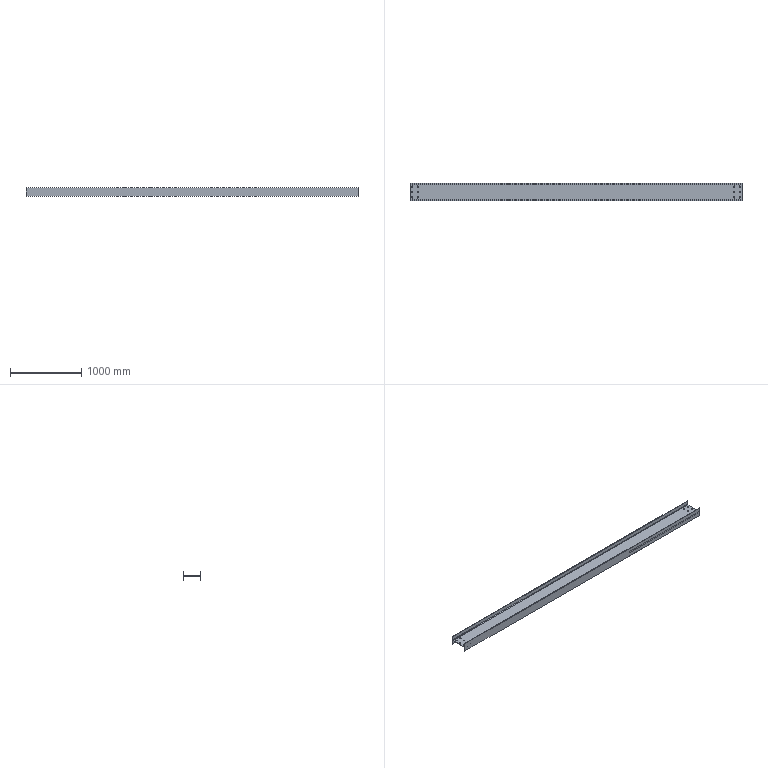Part | STEP file | 粉仓主梁6主体_Default<As Machined> | 1 solid | 42 faces | box 4655 x 250 x 125 mm | volume 17188833 mm3 | cylinder 28 | plane 14 | commonest cylinder face diameters 19 x24 16 x4